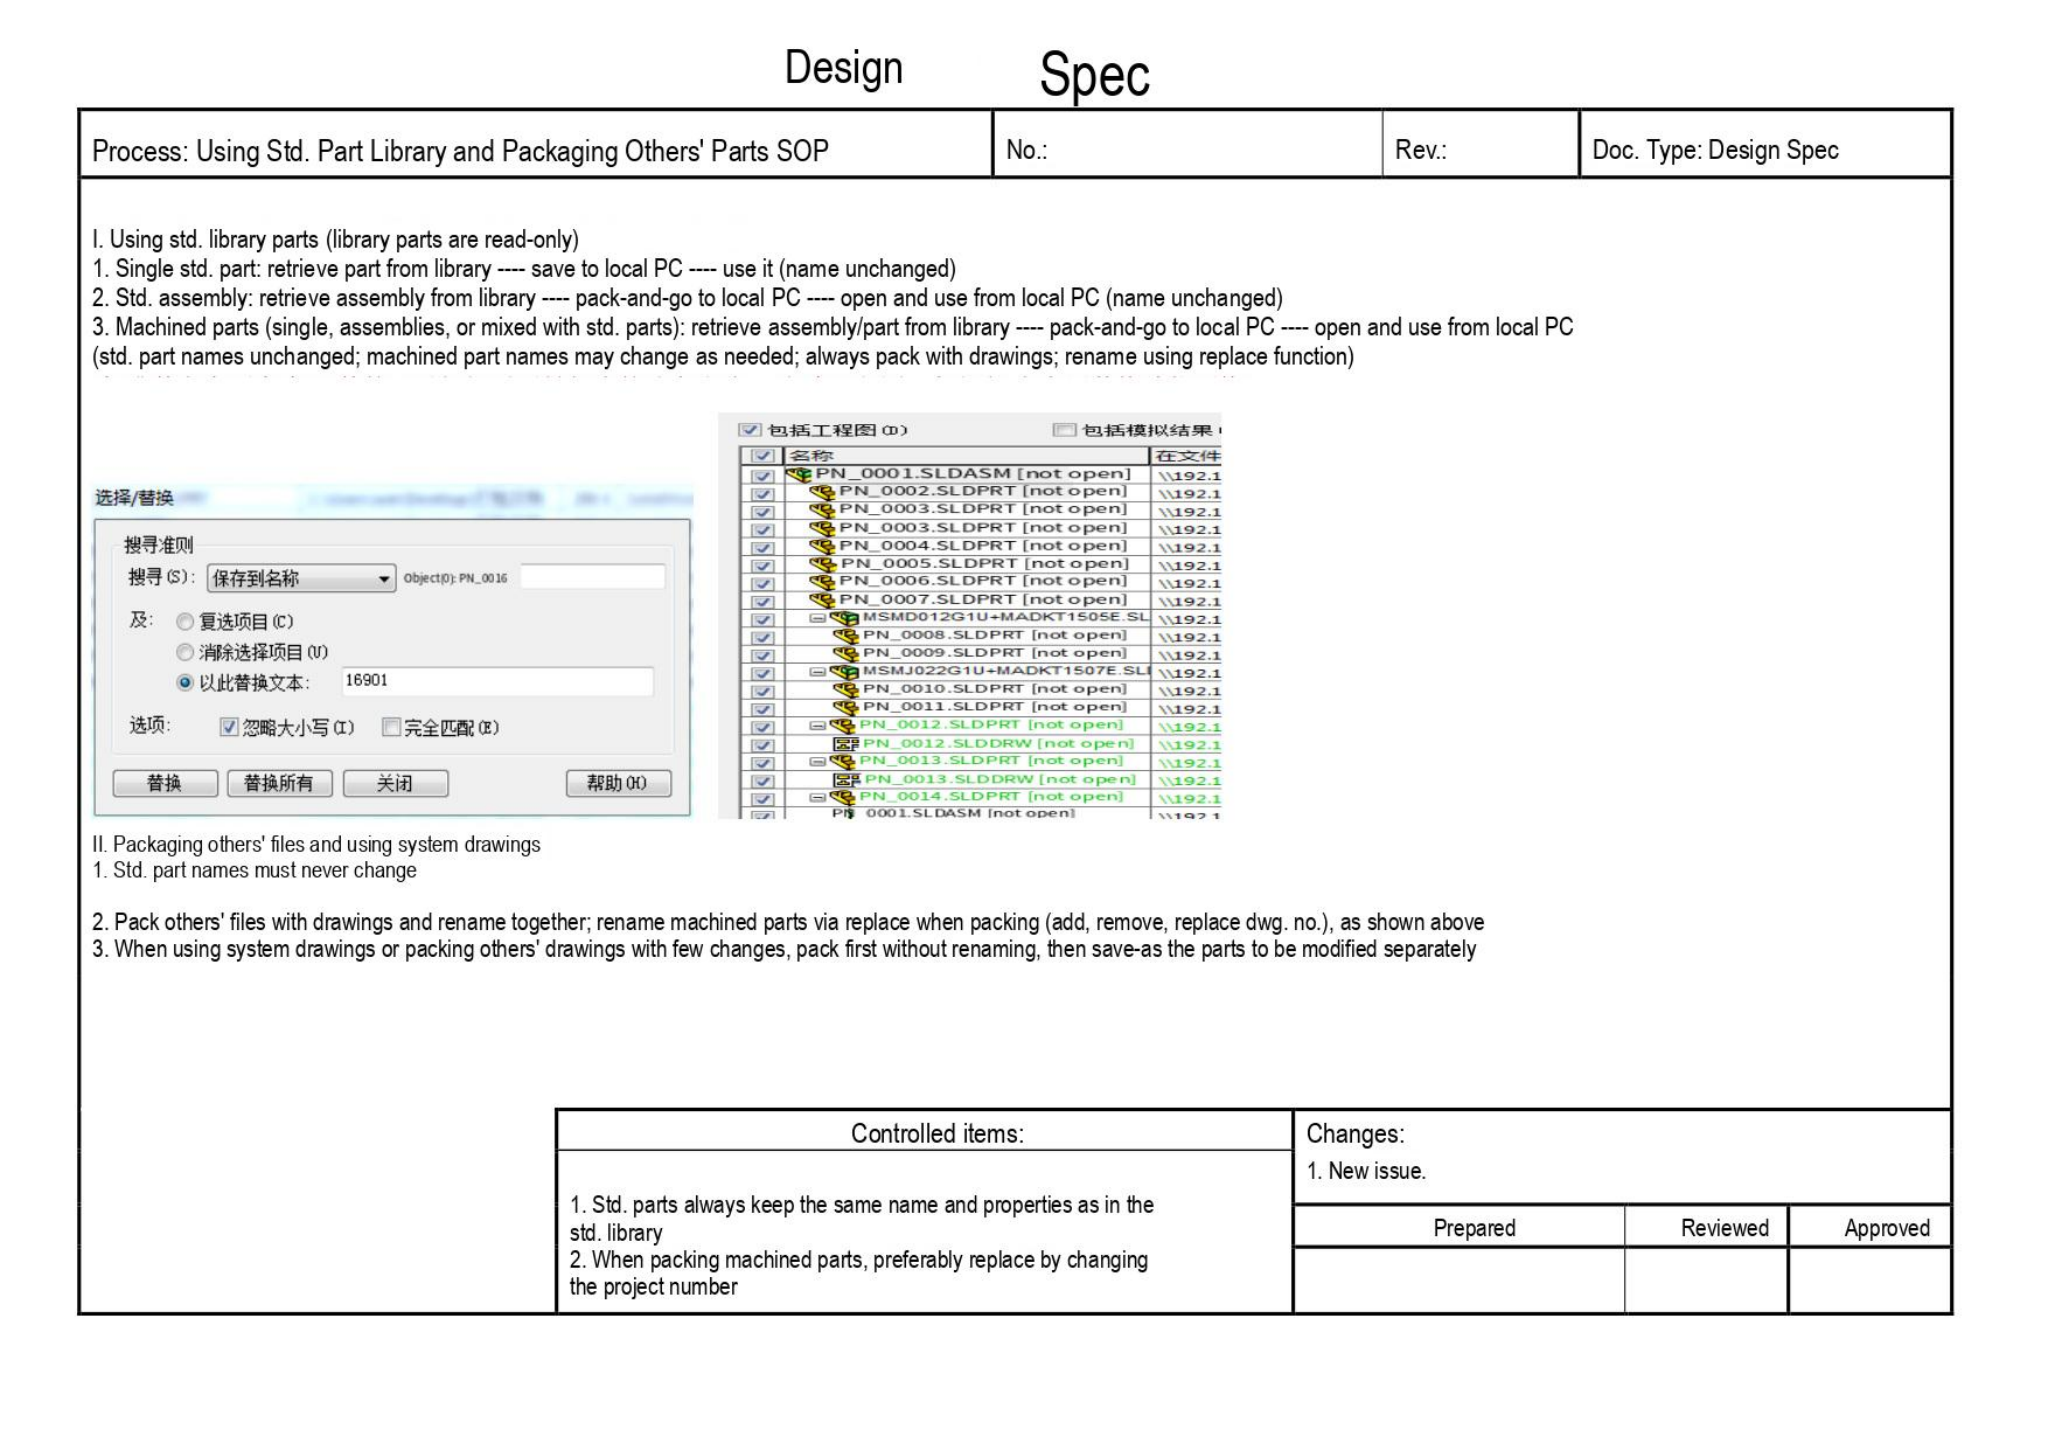Design Spec

| Process: Using Std. Part Library and Packaging Others' Parts SOP | No.: | Rev.: | Doc. Type: Design Spec |
|---|---|---|---|

I. Using std. library parts (library parts are read-only)
1. Single std. part: retrieve part from library ---- save to local PC ---- use it (name unchanged)
2. Std. assembly: retrieve assembly from library ---- pack-and-go to local PC ---- open and use from local PC (name unchanged)
3. Machined parts (single, assemblies, or mixed with std. parts): retrieve assembly/part from library ---- pack-and-go to local PC ---- open and use from local PC (std. part names unchanged; machined part names may change as needed; always pack with drawings; rename using replace function)

选择/替换
搜寻准则
搜寻 (S): 保存到名称 Object(0): PN_0016
及: 复选项目 (C)
消除选择项目 (U)
以此替换文本: 16901
选项: 忽略大小写 (I) 完全匹配 (E)
替换 替换所有 关闭 帮助 (H)

包括工程图 (D) 包括模拟结果

| 名称 | 在文件 |
|---|---|
| PN_0001.SLDASM [not open] | \\192.1 |
| PN_0002.SLDPRT [not open] | \\192.1 |
| PN_0003.SLDPRT [not open] | \\192.1 |
| PN_0003.SLDPRT [not open] | \\192.1 |
| PN_0004.SLDPRT [not open] | \\192.1 |
| PN_0005.SLDPRT [not open] | \\192.1 |
| PN_0006.SLDPRT [not open] | \\192.1 |
| PN_0007.SLDPRT [not open] | \\192.1 |
| MSMD012G1U+MADKT1505E.SL | \\192.1 |
| PN_0008.SLDPRT [not open] | \\192.1 |
| PN_0009.SLDPRT [not open] | \\192.1 |
| MSMJ022G1U+MADKT1507E.SL | \\192.1 |
| PN_0010.SLDPRT [not open] | \\192.1 |
| PN_0011.SLDPRT [not open] | \\192.1 |
| PN_0012.SLDPRT [not open] | \\192.1 |
| PN_0012.SLDDRW [not open] | \\192.1 |
| PN_0013.SLDPRT [not open] | \\192.1 |
| PN_0013.SLDDRW [not open] | \\192.1 |
| PN_0014.SLDPRT [not open] | \\192.1 |
| PN_0001.SLDASM [not open] | \\192.1 |

II. Packaging others' files and using system drawings
1. Std. part names must never change

2. Pack others' files with drawings and rename together; rename machined parts via replace when packing (add, remove, replace dwg. no.), as shown above
3. When using system drawings or packing others' drawings with few changes, pack first without renaming, then save-as the parts to be modified separately

| Controlled items: | Changes: 1. New issue. | | |
|---|---|---|---|
| 1. Std. parts always keep the same name and properties as in the std. library<br>2. When packing machined parts, preferably replace by changing the project number | Prepared | Reviewed | Approved |
| | | | |